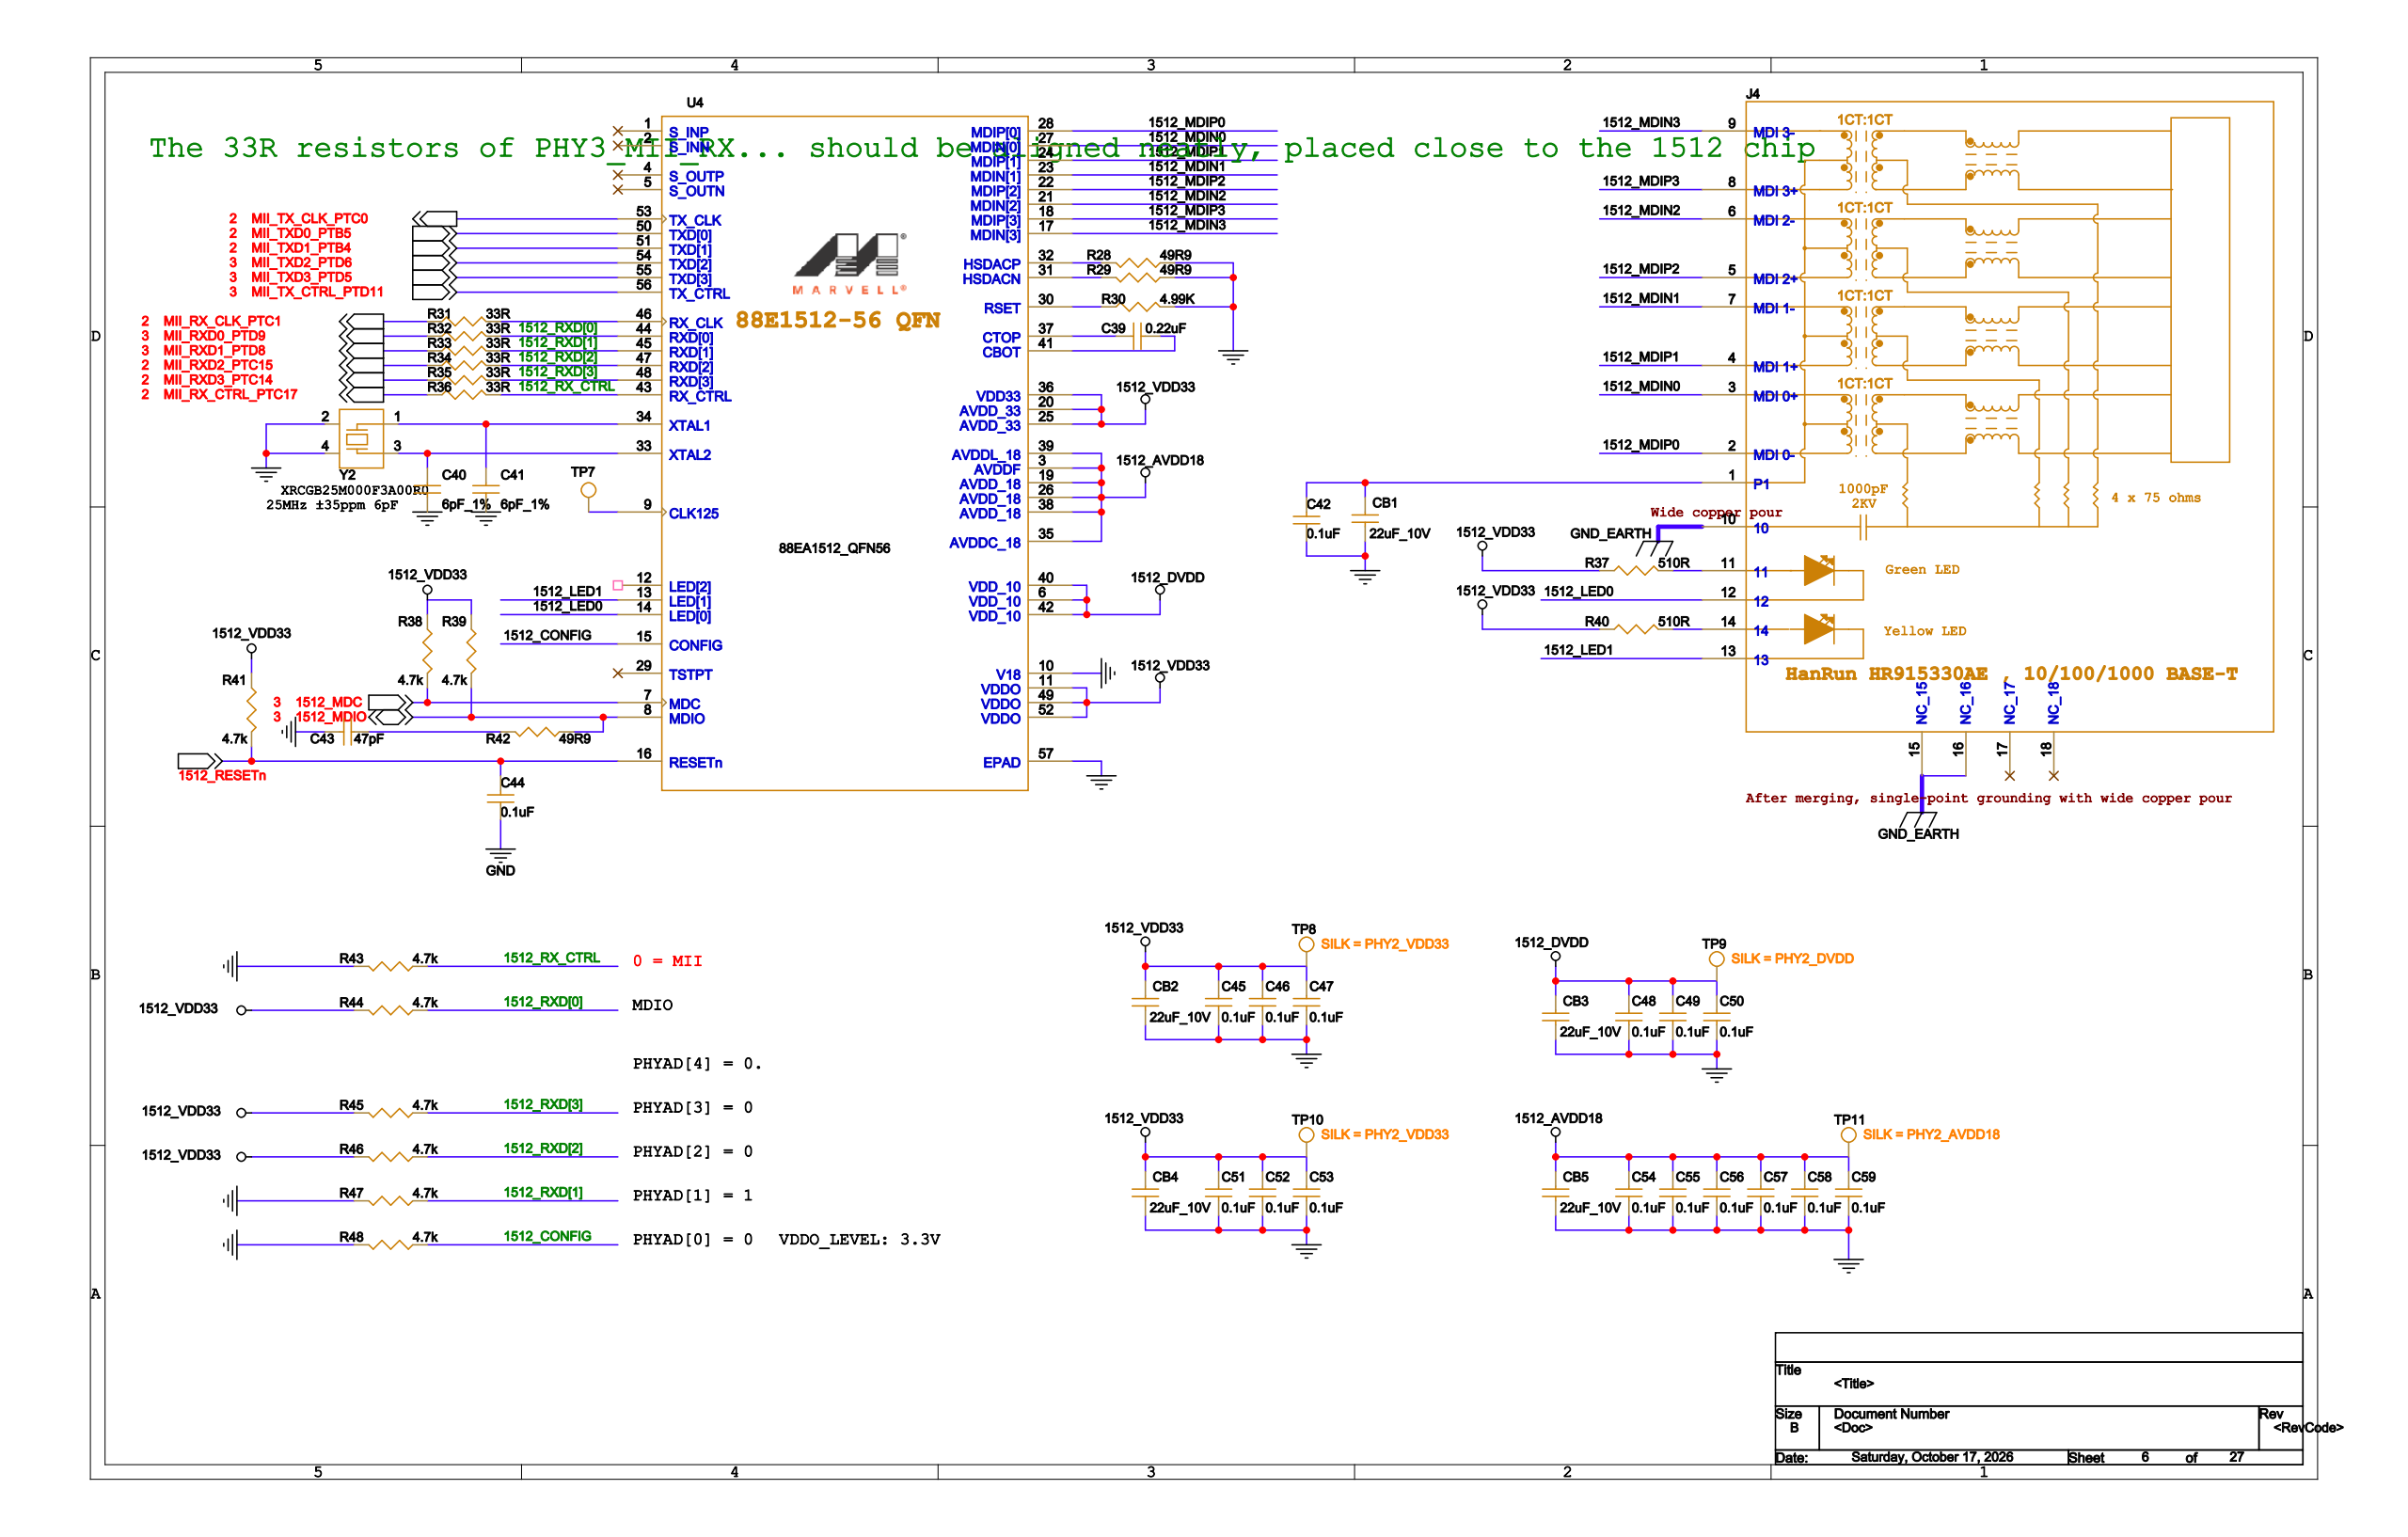Circuit board | Cadence Allegro | 477 parts | 327 nets | one sheet of the schematic
Parts on this sheet (reference | value | footprint):
C39 | 0.22uF | 0402
C40 | 6pF_1% | 0402
C41 | 6pF_1% | 0402
C42 | 0.1uF | 0402
C43 | 47pF | 0402
C44 | 0.1uF | 0402
C45 | 0.1uF | 0402
C46 | 0.1uF | 0402
C47 | 0.1uF | 0402
C48 | 0.1uF | 0402
C49 | 0.1uF | 0402
C50 | 0.1uF | 0402
C51 | 0.1uF | 0402
C52 | 0.1uF | 0402
C53 | 0.1uF | 0402
C54 | 0.1uF | 0402
C55 | 0.1uF | 0402
C56 | 0.1uF | 0402
C57 | 0.1uF | 0402
C58 | 0.1uF | 0402
C59 | 0.1uF | 0402
CB1 | 22uF_10V | 0805
CB2 | 22uF_10V | 0805
CB3 | 22uF_10V | 0805
CB4 | 22uF_10V | 0805
CB5 | 22uF_10V | 0805
J4 | HR915330AE | HR915330AE
R28 | 49R9 | 0402
R29 | 49R9 | 0402
R30 | 4.99K | 0402
R31 | 33R | 0402
R32 | 33R | 0402
R33 | 33R | 0402
R34 | 33R | 0402
R35 | 33R | 0402
R36 | 33R | 0402
R37 | 510R | 0402
R38 | 4.7K | 0402
R39 | 4.7K | 0402
R40 | 510R | 0402
R41 | 4.7K | 0402
R42 | 49R9 | 0402
R43 | 4.7K | 0402
R44 | 4.7K | 0402
R45 | 4.7K | 0402
R46 | 4.7K | 0402
R47 | 4.7K | 0402
R48 | 4.7K | 0402
TP7 | TP | S0400CI
TP8 | TP | S0400CI
TP9 | TP | S0400CI
TP10 | TP | S0400CI
TP11 | TP | S0400CI
U4 | 88EA1512_QFN56 | QFN50P800X800X100-56N_180X180EP
Y2 | XRCGB25M000F3A00R00 | CRYSTAL_SM
Nets of these parts (net: part-pin ...):
MII_TX_CTRL_PTD11: U4-56
MII_TXD3_PTD5: U4-55
MII_TXD2_PTD6: U4-54
MII_RX_CLK_PTC1: R31-1
N1754617: R31-2 U4-46
MII_RXD0_PTD9: R32-1
1512_RXD[0]: R32-2 R44-2 U4-44
MII_RXD1_PTD8: R33-1
1512_RXD[1]: R33-2 R47-2 U4-45
MII_RXD2_PTC15: R34-1
1512_RXD[2]: R34-2 R46-2 U4-47
MII_RXD3_PTC14: R35-1
1512_RXD[3]: R35-2 R45-2 U4-48
MII_RX_CTRL_PTC17: R36-1
1512_RX_CTRL: R36-2 R43-2 U4-43
MII_TXD1_PTB4: U4-51
MII_TXD0_PTB5: U4-50
MII_TX_CLK_PTC0: U4-53
GND: C40-2 C41-2 C42-1 C43-2 C44-1 C45-2 C46-2 C47-2 C48-2 C49-2 C50-2 C51-2 C52-2 C53-2 C54-2 C55-2 C56-2 C57-2 C58-2 C59-2 CB1-2 CB2-2 CB3-2 CB4-2 CB5-2 R28-2 R29-2 R30-2 R43-1 R47-1 R48-1 Y2-2 Y2-4 U4-10 U4-57
1512_MDC: R38-1 U4-7
1512_VDD33: C45-1 C46-1 C47-1 C51-1 C52-1 C53-1 CB2-1 CB4-1 R37-1 R38-2 R39-2 R40-1 R41-2 R44-1 R45-1 R46-1 TP8-1 TP10-1 U4-11 U4-20 U4-25 U4-36 U4-49 U4-52
1512_MDIO: R39-1 R42-2 U4-8
1512_RESETN: C44-2 R41-1 U4-16
1512_CONFIG: R48-2 U4-15
N1754463: R28-1 U4-32
N1754505: R29-1 U4-31
N1755361: C43-1 R42-1
N1754569: R30-1 U4-30
N1755135: J4-11 R37-2
N1755225: J4-14 R40-2
N1754891: C40-1 Y2-3 U4-33
N1754871: C41-1 Y2-1 U4-34
N1754991: C42-2 CB1-1 J4-1
1512_DVDD: C48-1 C49-1 C50-1 CB3-1 TP9-1 U4-6 U4-40 U4-42
1512_AVDD18: C54-1 C55-1 C56-1 C57-1 C58-1 C59-1 CB5-1 TP11-1 U4-3 U4-19 U4-26 U4-35 U4-38 U4-39
GND_EARTH: J4-10 J4-15 J4-16
1512_LED0: J4-12 U4-14
1512_LED1: J4-13 U4-13
1512_MDIN0: J4-3 U4-27
1512_MDIP0: J4-2 U4-28
1512_MDIP1: J4-4 U4-24
1512_MDIN1: J4-7 U4-23
1512_MDIP2: J4-5 U4-22
1512_MDIN2: J4-6 U4-21
1512_MDIP3: J4-8 U4-18
1512_MDIN3: J4-9 U4-17
N1754677: C39-2 U4-41
N1755027: TP7-1 U4-9
N1754673: C39-1 U4-37